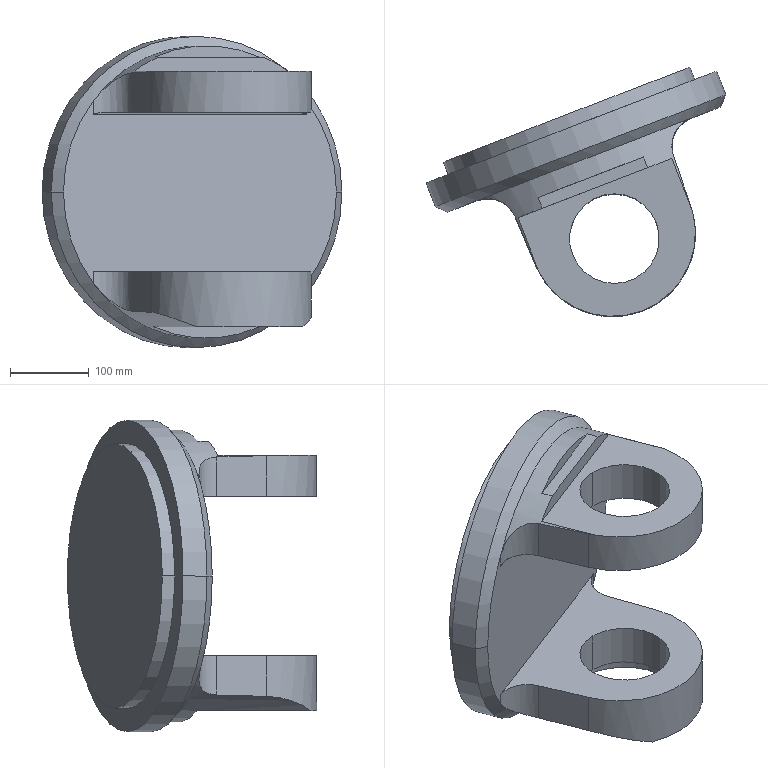Part | SolidWorks | features MoveFace 2, BaseBody 1, Scale 1 | 1 solid | 37 faces | box 381.228 x 317.121 x 396 mm | volume 10472227 mm3 | cylinder 19 | plane 16 | cone 2 | commonest cylinder face diameters 75.6 x4 114 x4 141.6 x2 211.33 x2 336 x2 372 x2